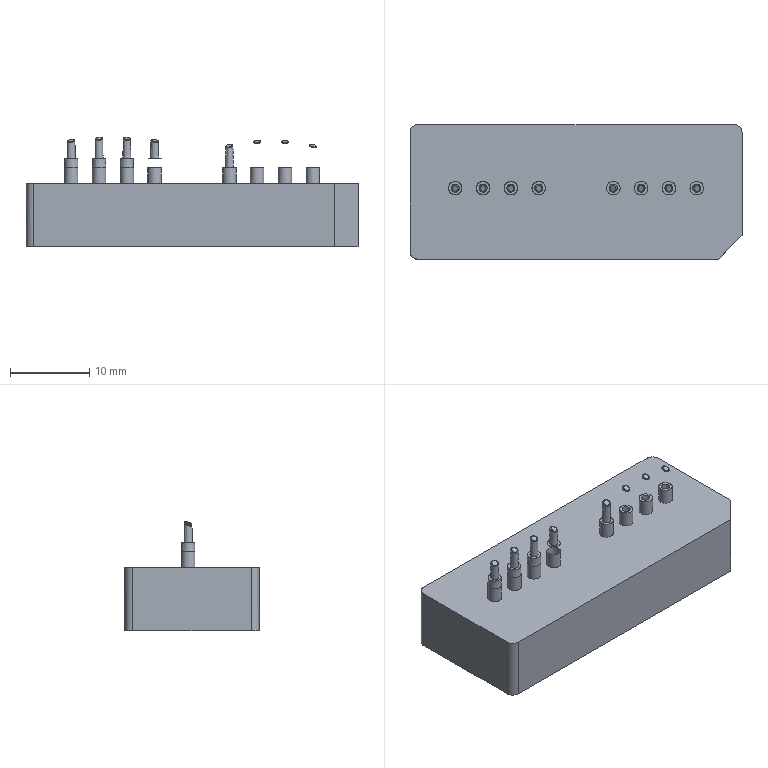CAM job | PowerMill | 3-axis milling, other | part box 42 x 17 x 13.856 mm
Tools:
number,name,type,diameter,tip_radius,length,cutting_length,overhang,flutes,holder,toolpaths_using
1,D10C,end_mill,10.0,0.0,60.0,,30.0,1,D42L35,1
15,D3C,end_mill,3.0,0.0,30.0,,15.0,1,D42L35,1
1,D10C_1_1,end_mill,10.0,0.0,60.0,,14.32,1,D42L35,3
15,D3C_1_1,end_mill,3.0,0.0,30.0,,6.04,1,D42L35,1
26,D1.5C_1_1,end_mill,1.5,0.0,4.84,,6.02,1,D42L35,1
3,D10_1_1,end_mill,10.0,0.0,60.0,,14.0,1,D42L35,2
6,R0.5_1_1,ball_nosed,1.0,0.5,3.0,,2.2,1,D42L35,1
20,D1.5_1_1,end_mill,1.5,0.0,4.88,,6.02,1,D42L35,1
13,Text_D4_1_1,taper_spherical,4.0,0.3,60.0,,6.12,1,D42L35,1
Operations:
program,toolpath,strategy,tool,tool_number,tool_diameter,tip_radius,flutes,spindle_rpm,feed_cut,surface_speed_m_min_computed,feed_per_tooth_computed,tolerance,thickness,stepover,stepdown,cut_length,cut_time_min,total_time_min,workplane
03-B01-2-F,精公开粗01-扫面平行-D10C,raster_area_clear,D10C_1_1,1,10.0,0.0,1.0,8000.0,10000.0,251.33,1.25,0.03,0.3,6.0,1.0,260.6,0.026,0.0323,
03-B01-2-F,精公开粗01-外形偏置-D10C,offset_area_clear,D10C_1_1,1,10.0,0.0,1.0,8000.0,10000.0,251.33,1.25,0.03,0.3,6.0,1.0,3700.388,0.37,0.4087,
03-B01-2-F,精公开粗01-基准台等高-D10C,constantz,D10C_1_1,1,10.0,0.0,1.0,8000.0,10000.0,251.33,1.25,0.03,0.07,5.0,0.4,3229.055,0.323,0.3318,
03-B01-2-F,精公再粗02-外形偏置-D3C,offset_area_clear,D3C_1_1,15,3.0,0.0,1.0,18000.0,5000.0,169.65,0.2778,0.03,0.02,2.0,1.0,2989.277,0.598,0.6697,
03-B01-2-F,精公再粗03-外形偏置-D1.5C,offset_area_clear,D1.5C_1_1,26,1.5,0.0,1.0,20000.0,3000.0,94.25,0.15,0.03,0.02,0.7,1.0,2883.54,0.961,1.814,
03-B01-2-F,精公基准台01-基准面偏置-D10,offset_area_clear,D10_1_1,3,10.0,0.0,1.0,8500.0,600.0,267.04,0.0706,0.005,0.4,5.0,1.0,113.309,0.189,0.2294,
03-B01-2-F,精公基准台01-基准台侧光-D10,profile_area_clear,D10_1_1,3,10.0,0.0,1.0,8500.0,600.0,267.04,0.0706,0.005,0.0,0.08,1.0,293.234,0.489,0.5522,
03-B01-2-F,精公精光01-平行-R0.5,raster,R0.5_1_1,6,1.0,0.5,1.0,20000.0,1000.0,62.83,0.05,0.005,-0.055,0.02,1.0,1632.331,1.632,1.68,
03-B01-2-F,精公精光02-等高-D1.5,constantz,D1.5_1_1,20,1.5,0.0,1.0,20000.0,1500.0,94.25,0.075,0.005,-0.055,5.0,0.03,12199.774,8.133,9.345,
03-B01-2-F,精公刻字01-刻字-Text_D4,pattern,Text_D4_1_1,13,4.0,0.3,1.0,15000.0,1000.0,188.5,0.0667,0.005,0.0,5.0,1.0,72.242,0.072,0.0905,
,精公开粗01-外形偏置-D10C_Reference,offset_area_clear,D10C,1,10.0,0.0,1.0,8000.0,10000.0,251.33,1.25,0.03,0.3,6.0,1.0,9637.705,0.964,1.061,
,精公再粗02-外形偏置-D3C_Reference,offset_area_clear,D3C,15,3.0,0.0,1.0,18000.0,5000.0,169.65,0.2778,0.03,0.02,2.0,1.0,8663.797,1.733,1.939,